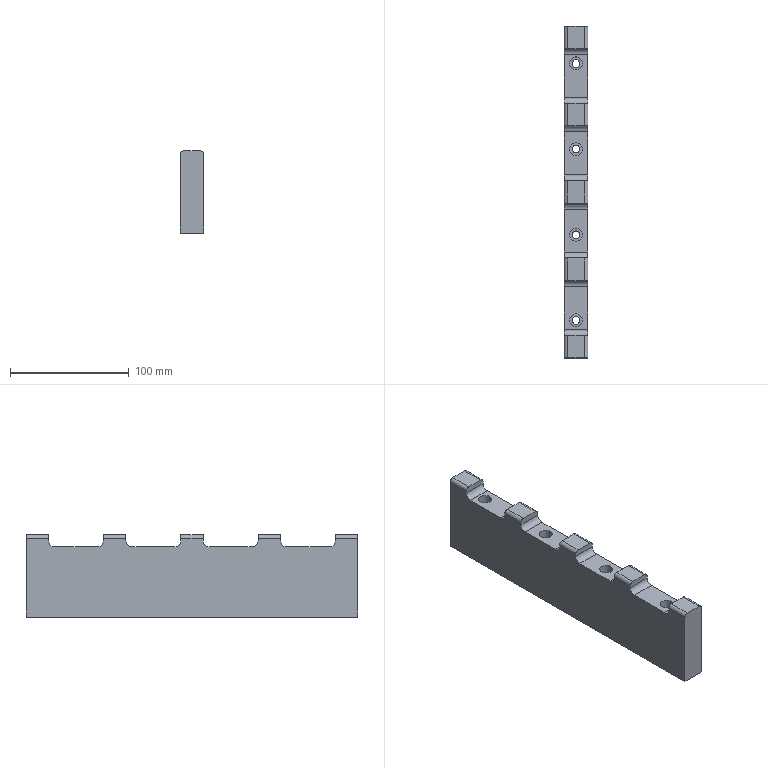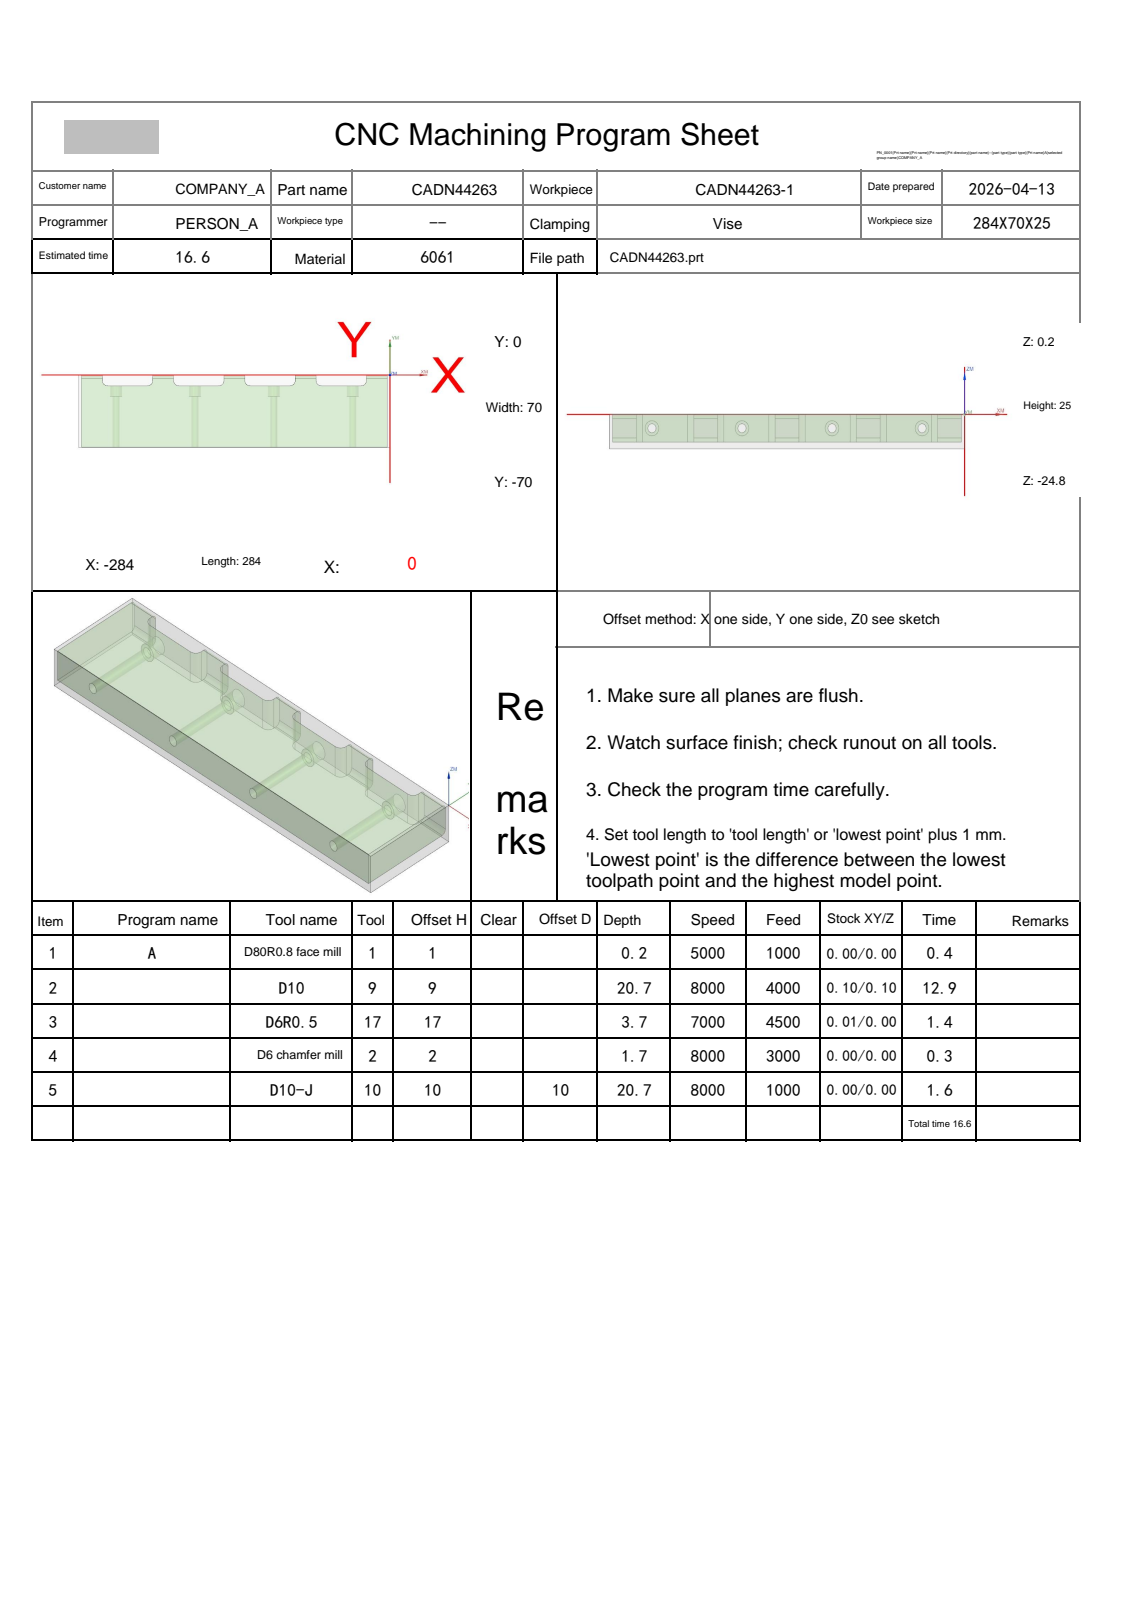NC program | NX | posted by the shop | part box 20 x 279 x 69 mm
Lines 1 to 31 of 9859:
%
O0001
(Machine time: 17.63 MIN)
(===Total Tool:5===)
(T1=D80R0.8 face mill D=80.  R=0.8  D-  H01 Z=-0.   )
(T9=D10     D=10.  R=0.   D-  H09 Z=-20.5 )
(T17=D6R0.5 D=6.   R=0.5  D-  H17 Z=-3.5  )
(T2=D6 chamfer mill   D=6.   R=0.   D-  H02 Z=-1.5  )
(T10=D10-J  D=10.  R=0.   D10 H10 Z=-20.5 )
G80 G90 G17 G49 G40
G91 G28 Z0
M01
N1 T01 M06
(D80R0.8 face mill  D=80. R=0.8 H=01 ce=0.00 di=0.00)
G00 G90 G54 X-326.5 Y-35. M03 S5000
G43 H01 Z20.
M08
Z2.
G01 Z0.0 F1000.
X-321.5
X37.5
X42.5
Z2.
G00 Z20.
G91 G28 Z0.0
M05
M09
G91 G28 Z0.0
M01